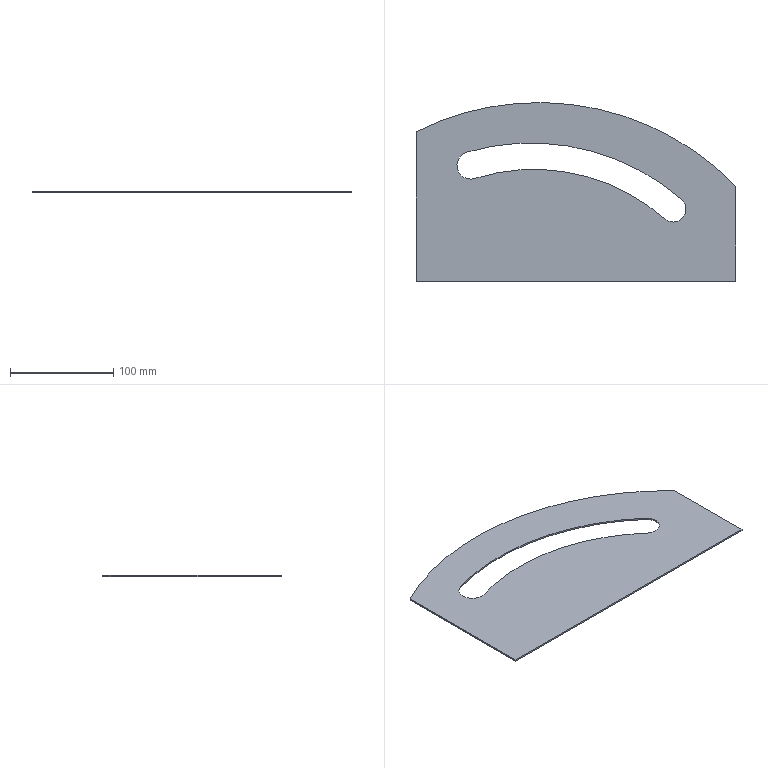Part | STEP file | DEWALT-DWE7492-B22 | 1 solid | 10 faces | box 310 x 173.249 x 1.5 mm | volume 62971 mm3 | cylinder 5 | plane 5 | commonest cylinder face diameters 25.007 x1 26.668 x1 381.573 x1 444.713 x1 530 x1
STEP:
#1=CARTESIAN_POINT('',(0.,0.,0.));
#2=DIRECTION('',(0.,0.,1.));
#3=DIRECTION('',(1.,0.,0.));
#4=AXIS2_PLACEMENT_3D('',#1,#2,#3);
#5=CARTESIAN_POINT('',(56.954,99.676,1.5));
#6=VERTEX_POINT('',#5);
#7=CARTESIAN_POINT('',(56.954,99.676,0.));
#8=VERTEX_POINT('',#7);
#9=CARTESIAN_POINT('',(56.954,99.676,1.5));
#10=DIRECTION('',(0.,0.,-1.));
#11=VECTOR('',#10,1.);
#12=LINE('',#9,#11);
#13=CARTESIAN_POINT('',(52.938,112.391,1.5));
#14=DIRECTION('',(0.,0.,-1.));
#15=DIRECTION('',(-1.,0.,0.));
#16=AXIS2_PLACEMENT_3D('',#13,#14,#15);
#17=CYLINDRICAL_SURFACE('',#16,13.334);
#18=CARTESIAN_POINT('',(4.406,0.));
#19=DIRECTION('',(0.,1.));
#20=VECTOR('',#19,1.);
#21=LINE('',#18,#20);
#22=(GEOMETRIC_REPRESENTATION_CONTEXT(2)PARAMETRIC_REPRESENTATION_CONTEXT()REPRESENTATION_CONTEXT('',''));
#23=DEFINITIONAL_REPRESENTATION('',(#21),#22);
#24=PCURVE('',#17,#23);
#25=CARTESIAN_POINT('',(114.412,-82.252,1.5));
#26=DIRECTION('',(0.,0.,-1.));
#27=DIRECTION('',(-1.,0.,0.));
#28=AXIS2_PLACEMENT_3D('',#25,#26,#27);
#29=CYLINDRICAL_SURFACE('',#28,190.787);
#30=CARTESIAN_POINT('',(1.265,0.));
#31=DIRECTION('',(0.,1.));
#32=VECTOR('',#31,1.);
#33=LINE('',#30,#32);
#34=(GEOMETRIC_REPRESENTATION_CONTEXT(2)PARAMETRIC_REPRESENTATION_CONTEXT()REPRESENTATION_CONTEXT('',''));
#35=DEFINITIONAL_REPRESENTATION('',(#33),#34);
#36=PCURVE('',#29,#35);
#37=SURFACE_CURVE('',#12,(#24,#36),.PCURVE_S1.);
#38=EDGE_CURVE('',#6,#8,#37,.T.);
#39=ORIENTED_EDGE('',*,*,#38,.F.);
#40=CARTESIAN_POINT('',(49.212,125.194,1.5));
#41=VERTEX_POINT('',#40);
#42=CARTESIAN_POINT('',(52.938,112.391,1.5));
#43=DIRECTION('',(0.,0.,-1.));
#44=DIRECTION('',(1.,0.,0.));
#45=AXIS2_PLACEMENT_3D('',#42,#43,#44);
#46=CIRCLE('',#45,13.334);
#47=CARTESIAN_POINT('',(3.142,0.));
#48=DIRECTION('',(1.,0.));
#49=VECTOR('',#48,1.);
#50=LINE('',#47,#49);
#51=(GEOMETRIC_REPRESENTATION_CONTEXT(2)PARAMETRIC_REPRESENTATION_CONTEXT()REPRESENTATION_CONTEXT('',''));
#52=DEFINITIONAL_REPRESENTATION('',(#50),#51);
#53=PCURVE('',#17,#52);
#54=CARTESIAN_POINT('',(119.054,-91.751,1.5));
#55=DIRECTION('',(0.,0.,-1.));
#56=DIRECTION('',(-1.,0.,0.));
#57=AXIS2_PLACEMENT_3D('',#54,#55,#56);
#58=PLANE('',#57);
#59=CARTESIAN_POINT('',(66.116,204.143));
#60=DIRECTION('',(-1.,0.));
#61=AXIS2_PLACEMENT_2D('',#59,#60);
#62=CIRCLE('',#61,13.334);
#63=(GEOMETRIC_REPRESENTATION_CONTEXT(2)PARAMETRIC_REPRESENTATION_CONTEXT()REPRESENTATION_CONTEXT('',''));
#64=DEFINITIONAL_REPRESENTATION('',(#62),#63);
#65=PCURVE('',#58,#64);
#66=SURFACE_CURVE('',#46,(#53,#65),.PCURVE_S1.);
#67=EDGE_CURVE('',#6,#41,#66,.T.);
#68=ORIENTED_EDGE('',*,*,#67,.T.);
#69=CARTESIAN_POINT('',(49.212,125.194,0.));
#70=VERTEX_POINT('',#69);
#71=CARTESIAN_POINT('',(49.212,125.194,1.5));
#72=DIRECTION('',(0.,0.,-1.));
#73=VECTOR('',#72,1.);
#74=LINE('',#71,#73);
#75=CARTESIAN_POINT('',(7.571,0.));
#76=DIRECTION('',(0.,1.));
#77=VECTOR('',#76,1.);
#78=LINE('',#75,#77);
#79=(GEOMETRIC_REPRESENTATION_CONTEXT(2)PARAMETRIC_REPRESENTATION_CONTEXT()REPRESENTATION_CONTEXT('',''));
#80=DEFINITIONAL_REPRESENTATION('',(#78),#79);
#81=PCURVE('',#17,#80);
#82=CARTESIAN_POINT('',(111.356,-88.302,1.5));
#83=DIRECTION('',(0.,0.,-1.));
#84=DIRECTION('',(-1.,0.,0.));
#85=AXIS2_PLACEMENT_3D('',#82,#83,#84);
#86=CYLINDRICAL_SURFACE('',#85,222.357);
#87=CARTESIAN_POINT('',(1.288,0.));
#88=DIRECTION('',(0.,1.));
#89=VECTOR('',#88,1.);
#90=LINE('',#87,#89);
#91=(GEOMETRIC_REPRESENTATION_CONTEXT(2)PARAMETRIC_REPRESENTATION_CONTEXT()REPRESENTATION_CONTEXT('',''));
#92=DEFINITIONAL_REPRESENTATION('',(#90),#91);
#93=PCURVE('',#86,#92);
#94=SURFACE_CURVE('',#74,(#81,#93),.PCURVE_S1.);
#95=EDGE_CURVE('',#41,#70,#94,.T.);
#96=ORIENTED_EDGE('',*,*,#95,.T.);
#97=CARTESIAN_POINT('',(52.938,112.391,0.));
#98=DIRECTION('',(0.,0.,-1.));
#99=DIRECTION('',(1.,0.,0.));
#100=AXIS2_PLACEMENT_3D('',#97,#98,#99);
#101=CIRCLE('',#100,13.334);
#102=CARTESIAN_POINT('',(3.142,1.5));
#103=DIRECTION('',(1.,0.));
#104=VECTOR('',#103,1.);
#105=LINE('',#102,#104);
#106=(GEOMETRIC_REPRESENTATION_CONTEXT(2)PARAMETRIC_REPRESENTATION_CONTEXT()REPRESENTATION_CONTEXT('',''));
#107=DEFINITIONAL_REPRESENTATION('',(#105),#106);
#108=PCURVE('',#17,#107);
#109=CARTESIAN_POINT('',(119.054,-91.751,0.));
#110=DIRECTION('',(0.,0.,-1.));
#111=DIRECTION('',(-1.,0.,0.));
#112=AXIS2_PLACEMENT_3D('',#109,#110,#111);
#113=PLANE('',#112);
#114=CARTESIAN_POINT('',(66.116,204.143));
#115=DIRECTION('',(-1.,0.));
#116=AXIS2_PLACEMENT_2D('',#114,#115);
#117=CIRCLE('',#116,13.334);
#118=(GEOMETRIC_REPRESENTATION_CONTEXT(2)PARAMETRIC_REPRESENTATION_CONTEXT()REPRESENTATION_CONTEXT('',''));
#119=DEFINITIONAL_REPRESENTATION('',(#117),#118);
#120=PCURVE('',#113,#119);
#121=SURFACE_CURVE('',#101,(#108,#120),.PCURVE_S1.);
#122=EDGE_CURVE('',#8,#70,#121,.T.);
#123=ORIENTED_EDGE('',*,*,#122,.F.);
#124=EDGE_LOOP('',(#39,#68,#96,#123));
#125=FACE_BOUND('',#124,.F.);
#126=ADVANCED_FACE('',(#125),#17,.F.);
#127=CARTESIAN_POINT('',(240.815,60.652,0.));
#128=VERTEX_POINT('',#127);
#129=CARTESIAN_POINT('',(114.412,-82.252,0.));
#130=DIRECTION('',(0.,0.,1.));
#131=DIRECTION('',(1.,0.,0.));
#132=AXIS2_PLACEMENT_3D('',#129,#130,#131);
#133=CIRCLE('',#132,190.787);
#134=CARTESIAN_POINT('',(3.142,1.5));
#135=DIRECTION('',(-1.,0.));
#136=VECTOR('',#135,1.);
#137=LINE('',#134,#136);
#138=(GEOMETRIC_REPRESENTATION_CONTEXT(2)PARAMETRIC_REPRESENTATION_CONTEXT()REPRESENTATION_CONTEXT('',''));
#139=DEFINITIONAL_REPRESENTATION('',(#137),#138);
#140=PCURVE('',#29,#139);
#141=CARTESIAN_POINT('',(-186.145,9.499));
#142=CARTESIAN_POINT('',(-186.145,339.951));
#143=CARTESIAN_POINT('',(100.035,174.725));
#144=CARTESIAN_POINT('',(386.215,9.499));
#145=CARTESIAN_POINT('',(100.035,-155.727));
#146=CARTESIAN_POINT('',(-186.145,-320.953));
#147=CARTESIAN_POINT('',(-186.145,9.499));
#148=(BOUNDED_CURVE()B_SPLINE_CURVE(2,(#141,#142,#143,#144,#145,#146,#147),.UNSPECIFIED.,.T.,.F.)B_SPLINE_CURVE_WITH_KNOTS((1,2,2,2,2,1),(-2.094,0.,2.094,4.189,6.283,8.378),.UNSPECIFIED.)CURVE()GEOMETRIC_REPRESENTATION_ITEM()RATIONAL_B_SPLINE_CURVE((1.,0.5,1.,0.5,1.,0.5,1.))REPRESENTATION_ITEM(''));
#149=(GEOMETRIC_REPRESENTATION_CONTEXT(2)PARAMETRIC_REPRESENTATION_CONTEXT()REPRESENTATION_CONTEXT('',''));
#150=DEFINITIONAL_REPRESENTATION('',(#148),#149);
#151=PCURVE('',#113,#150);
#152=SURFACE_CURVE('',#133,(#140,#151),.PCURVE_S1.);
#153=EDGE_CURVE('',#128,#8,#152,.T.);
#154=ORIENTED_EDGE('',*,*,#153,.T.);
#155=ORIENTED_EDGE('',*,*,#38,.F.);
#156=CARTESIAN_POINT('',(240.815,60.652,1.5));
#157=VERTEX_POINT('',#156);
#158=CARTESIAN_POINT('',(114.412,-82.252,1.5));
#159=DIRECTION('',(0.,0.,1.));
#160=DIRECTION('',(1.,0.,0.));
#161=AXIS2_PLACEMENT_3D('',#158,#159,#160);
#162=CIRCLE('',#161,190.787);
#163=CARTESIAN_POINT('',(3.142,0.));
#164=DIRECTION('',(-1.,0.));
#165=VECTOR('',#164,1.);
#166=LINE('',#163,#165);
#167=(GEOMETRIC_REPRESENTATION_CONTEXT(2)PARAMETRIC_REPRESENTATION_CONTEXT()REPRESENTATION_CONTEXT('',''));
#168=DEFINITIONAL_REPRESENTATION('',(#166),#167);
#169=PCURVE('',#29,#168);
#170=CARTESIAN_POINT('',(-186.145,9.499));
#171=CARTESIAN_POINT('',(-186.145,339.951));
#172=CARTESIAN_POINT('',(100.035,174.725));
#173=CARTESIAN_POINT('',(386.215,9.499));
#174=CARTESIAN_POINT('',(100.035,-155.727));
#175=CARTESIAN_POINT('',(-186.145,-320.953));
#176=CARTESIAN_POINT('',(-186.145,9.499));
#177=(BOUNDED_CURVE()B_SPLINE_CURVE(2,(#170,#171,#172,#173,#174,#175,#176),.UNSPECIFIED.,.T.,.F.)B_SPLINE_CURVE_WITH_KNOTS((1,2,2,2,2,1),(-2.094,0.,2.094,4.189,6.283,8.378),.UNSPECIFIED.)CURVE()GEOMETRIC_REPRESENTATION_ITEM()RATIONAL_B_SPLINE_CURVE((1.,0.5,1.,0.5,1.,0.5,1.))REPRESENTATION_ITEM(''));
#178=(GEOMETRIC_REPRESENTATION_CONTEXT(2)PARAMETRIC_REPRESENTATION_CONTEXT()REPRESENTATION_CONTEXT('',''));
#179=DEFINITIONAL_REPRESENTATION('',(#177),#178);
#180=PCURVE('',#58,#179);
#181=SURFACE_CURVE('',#162,(#169,#180),.PCURVE_S1.);
#182=EDGE_CURVE('',#157,#6,#181,.T.);
#183=ORIENTED_EDGE('',*,*,#182,.F.);
#184=CARTESIAN_POINT('',(240.815,60.652,1.5));
#185=DIRECTION('',(0.,0.,-1.));
#186=VECTOR('',#185,1.);
#187=LINE('',#184,#186);
#188=CARTESIAN_POINT('',(2.295,0.));
#189=DIRECTION('',(0.,1.));
#190=VECTOR('',#189,1.);
#191=LINE('',#188,#190);
#192=(GEOMETRIC_REPRESENTATION_CONTEXT(2)PARAMETRIC_REPRESENTATION_CONTEXT()REPRESENTATION_CONTEXT('',''));
#193=DEFINITIONAL_REPRESENTATION('',(#191),#192);
#194=PCURVE('',#29,#193);
#195=CARTESIAN_POINT('',(249.099,70.018,1.5));
#196=DIRECTION('',(0.,0.,-1.));
#197=DIRECTION('',(-1.,0.,0.));
#198=AXIS2_PLACEMENT_3D('',#195,#196,#197);
#199=CYLINDRICAL_SURFACE('',#198,12.504);
#200=CARTESIAN_POINT('',(5.437,0.));
#201=DIRECTION('',(0.,1.));
#202=VECTOR('',#201,1.);
#203=LINE('',#200,#202);
#204=(GEOMETRIC_REPRESENTATION_CONTEXT(2)PARAMETRIC_REPRESENTATION_CONTEXT()REPRESENTATION_CONTEXT('',''));
#205=DEFINITIONAL_REPRESENTATION('',(#203),#204);
#206=PCURVE('',#199,#205);
#207=SURFACE_CURVE('',#187,(#194,#206),.PCURVE_S1.);
#208=EDGE_CURVE('',#157,#128,#207,.T.);
#209=ORIENTED_EDGE('',*,*,#208,.T.);
#210=EDGE_LOOP('',(#154,#155,#183,#209));
#211=FACE_BOUND('',#210,.T.);
#212=ADVANCED_FACE('',(#211),#29,.T.);
#213=CARTESIAN_POINT('',(257.306,79.451,1.5));
#214=VERTEX_POINT('',#213);
#215=CARTESIAN_POINT('',(257.306,79.451,0.));
#216=VERTEX_POINT('',#215);
#217=CARTESIAN_POINT('',(257.306,79.451,1.5));
#218=DIRECTION('',(0.,0.,-1.));
#219=VECTOR('',#218,1.);
#220=LINE('',#217,#219);
#221=CARTESIAN_POINT('',(2.287,0.));
#222=DIRECTION('',(0.,1.));
#223=VECTOR('',#222,1.);
#224=LINE('',#221,#223);
#225=(GEOMETRIC_REPRESENTATION_CONTEXT(2)PARAMETRIC_REPRESENTATION_CONTEXT()REPRESENTATION_CONTEXT('',''));
#226=DEFINITIONAL_REPRESENTATION('',(#224),#225);
#227=PCURVE('',#199,#226);
#228=CARTESIAN_POINT('',(2.287,0.));
#229=DIRECTION('',(0.,1.));
#230=VECTOR('',#229,1.);
#231=LINE('',#228,#230);
#232=(GEOMETRIC_REPRESENTATION_CONTEXT(2)PARAMETRIC_REPRESENTATION_CONTEXT()REPRESENTATION_CONTEXT('',''));
#233=DEFINITIONAL_REPRESENTATION('',(#231),#232);
#234=PCURVE('',#86,#233);
#235=SURFACE_CURVE('',#220,(#227,#234),.PCURVE_S1.);
#236=EDGE_CURVE('',#214,#216,#235,.T.);
#237=ORIENTED_EDGE('',*,*,#236,.F.);
#238=CARTESIAN_POINT('',(249.099,70.018,1.5));
#239=DIRECTION('',(0.,0.,-1.));
#240=DIRECTION('',(-1.,0.,0.));
#241=AXIS2_PLACEMENT_3D('',#238,#239,#240);
#242=CIRCLE('',#241,12.504);
#243=CARTESIAN_POINT('',(0.,0.));
#244=DIRECTION('',(1.,0.));
#245=VECTOR('',#244,1.);
#246=LINE('',#243,#245);
#247=(GEOMETRIC_REPRESENTATION_CONTEXT(2)PARAMETRIC_REPRESENTATION_CONTEXT()REPRESENTATION_CONTEXT('',''));
#248=DEFINITIONAL_REPRESENTATION('',(#246),#247);
#249=PCURVE('',#199,#248);
#250=CARTESIAN_POINT('',(-130.045,161.769));
#251=DIRECTION('',(1.,0.));
#252=AXIS2_PLACEMENT_2D('',#250,#251);
#253=CIRCLE('',#252,12.504);
#254=(GEOMETRIC_REPRESENTATION_CONTEXT(2)PARAMETRIC_REPRESENTATION_CONTEXT()REPRESENTATION_CONTEXT('',''));
#255=DEFINITIONAL_REPRESENTATION('',(#253),#254);
#256=PCURVE('',#58,#255);
#257=SURFACE_CURVE('',#242,(#249,#256),.PCURVE_S1.);
#258=EDGE_CURVE('',#214,#157,#257,.T.);
#259=ORIENTED_EDGE('',*,*,#258,.T.);
#260=ORIENTED_EDGE('',*,*,#208,.T.);
#261=CARTESIAN_POINT('',(249.099,70.018,0.));
#262=DIRECTION('',(0.,0.,-1.));
#263=DIRECTION('',(-1.,0.,0.));
#264=AXIS2_PLACEMENT_3D('',#261,#262,#263);
#265=CIRCLE('',#264,12.504);
#266=CARTESIAN_POINT('',(0.,1.5));
#267=DIRECTION('',(1.,0.));
#268=VECTOR('',#267,1.);
#269=LINE('',#266,#268);
#270=(GEOMETRIC_REPRESENTATION_CONTEXT(2)PARAMETRIC_REPRESENTATION_CONTEXT()REPRESENTATION_CONTEXT('',''));
#271=DEFINITIONAL_REPRESENTATION('',(#269),#270);
#272=PCURVE('',#199,#271);
#273=CARTESIAN_POINT('',(-130.045,161.769));
#274=DIRECTION('',(1.,0.));
#275=AXIS2_PLACEMENT_2D('',#273,#274);
#276=CIRCLE('',#275,12.504);
#277=(GEOMETRIC_REPRESENTATION_CONTEXT(2)PARAMETRIC_REPRESENTATION_CONTEXT()REPRESENTATION_CONTEXT('',''));
#278=DEFINITIONAL_REPRESENTATION('',(#276),#277);
#279=PCURVE('',#113,#278);
#280=SURFACE_CURVE('',#265,(#272,#279),.PCURVE_S1.);
#281=EDGE_CURVE('',#216,#128,#280,.T.);
#282=ORIENTED_EDGE('',*,*,#281,.F.);
#283=EDGE_LOOP('',(#237,#259,#260,#282));
#284=FACE_BOUND('',#283,.F.);
#285=ADVANCED_FACE('',(#284),#199,.F.);
#286=CARTESIAN_POINT('',(310.,0.,0.));
#287=VERTEX_POINT('',#286);
#288=CARTESIAN_POINT('',(0.,0.,0.));
#289=VERTEX_POINT('',#288);
#290=CARTESIAN_POINT('',(310.,0.,0.));
#291=DIRECTION('',(-1.,0.,0.));
#292=VECTOR('',#291,1.);
#293=LINE('',#290,#292);
#294=CARTESIAN_POINT('',(310.,0.,1.5));
#295=DIRECTION('',(0.,-1.,0.));
#296=DIRECTION('',(0.,0.,-1.));
#297=AXIS2_PLACEMENT_3D('',#294,#295,#296);
#298=PLANE('',#297);
#299=CARTESIAN_POINT('',(1.5,0.));
#300=DIRECTION('',(0.,-1.));
#301=VECTOR('',#300,1.);
#302=LINE('',#299,#301);
#303=(GEOMETRIC_REPRESENTATION_CONTEXT(2)PARAMETRIC_REPRESENTATION_CONTEXT()REPRESENTATION_CONTEXT('',''));
#304=DEFINITIONAL_REPRESENTATION('',(#302),#303);
#305=PCURVE('',#298,#304);
#306=CARTESIAN_POINT('',(-190.946,91.751));
#307=DIRECTION('',(1.,0.));
#308=VECTOR('',#307,1.);
#309=LINE('',#306,#308);
#310=(GEOMETRIC_REPRESENTATION_CONTEXT(2)PARAMETRIC_REPRESENTATION_CONTEXT()REPRESENTATION_CONTEXT('',''));
#311=DEFINITIONAL_REPRESENTATION('',(#309),#310);
#312=PCURVE('',#113,#311);
#313=SURFACE_CURVE('',#293,(#305,#312),.PCURVE_S1.);
#314=EDGE_CURVE('',#287,#289,#313,.T.);
#315=ORIENTED_EDGE('',*,*,#314,.F.);
#316=CARTESIAN_POINT('',(310.,0.,1.5));
#317=VERTEX_POINT('',#316);
#318=CARTESIAN_POINT('',(310.,0.,1.5));
#319=DIRECTION('',(0.,0.,-1.));
#320=VECTOR('',#319,1.);
#321=LINE('',#318,#320);
#322=CARTESIAN_POINT('',(0.,0.));
#323=DIRECTION('',(1.,0.));
#324=VECTOR('',#323,1.);
#325=LINE('',#322,#324);
#326=(GEOMETRIC_REPRESENTATION_CONTEXT(2)PARAMETRIC_REPRESENTATION_CONTEXT()REPRESENTATION_CONTEXT('',''));
#327=DEFINITIONAL_REPRESENTATION('',(#325),#326);
#328=PCURVE('',#298,#327);
#329=CARTESIAN_POINT('',(310.,92.,1.5));
#330=DIRECTION('',(1.,0.,0.));
#331=DIRECTION('',(0.,0.,-1.));
#332=AXIS2_PLACEMENT_3D('',#329,#330,#331);
#333=PLANE('',#332);
#334=CARTESIAN_POINT('',(0.,-92.));
#335=DIRECTION('',(1.,0.));
#336=VECTOR('',#335,1.);
#337=LINE('',#334,#336);
#338=(GEOMETRIC_REPRESENTATION_CONTEXT(2)PARAMETRIC_REPRESENTATION_CONTEXT()REPRESENTATION_CONTEXT('',''));
#339=DEFINITIONAL_REPRESENTATION('',(#337),#338);
#340=PCURVE('',#333,#339);
#341=SURFACE_CURVE('',#321,(#328,#340),.PCURVE_S1.);
#342=EDGE_CURVE('',#317,#287,#341,.T.);
#343=ORIENTED_EDGE('',*,*,#342,.F.);
#344=CARTESIAN_POINT('',(0.,0.,1.5));
#345=VERTEX_POINT('',#344);
#346=CARTESIAN_POINT('',(310.,0.,1.5));
#347=DIRECTION('',(-1.,0.,0.));
#348=VECTOR('',#347,1.);
#349=LINE('',#346,#348);
#350=CARTESIAN_POINT('',(0.,0.));
#351=DIRECTION('',(0.,-1.));
#352=VECTOR('',#351,1.);
#353=LINE('',#350,#352);
#354=(GEOMETRIC_REPRESENTATION_CONTEXT(2)PARAMETRIC_REPRESENTATION_CONTEXT()REPRESENTATION_CONTEXT('',''));
#355=DEFINITIONAL_REPRESENTATION('',(#353),#354);
#356=PCURVE('',#298,#355);
#357=CARTESIAN_POINT('',(-190.946,91.751));
#358=DIRECTION('',(1.,0.));
#359=VECTOR('',#358,1.);
#360=LINE('',#357,#359);
#361=(GEOMETRIC_REPRESENTATION_CONTEXT(2)PARAMETRIC_REPRESENTATION_CONTEXT()REPRESENTATION_CONTEXT('',''));
#362=DEFINITIONAL_REPRESENTATION('',(#360),#361);
#363=PCURVE('',#58,#362);
#364=SURFACE_CURVE('',#349,(#356,#363),.PCURVE_S1.);
#365=EDGE_CURVE('',#317,#345,#364,.T.);
#366=ORIENTED_EDGE('',*,*,#365,.T.);
#367=CARTESIAN_POINT('',(0.,0.,1.5));
#368=DIRECTION('',(0.,0.,-1.));
#369=VECTOR('',#368,1.);
#370=LINE('',#367,#369);
#371=CARTESIAN_POINT('',(0.,-310.));
#372=DIRECTION('',(1.,0.));
#373=VECTOR('',#372,1.);
#374=LINE('',#371,#373);
#375=(GEOMETRIC_REPRESENTATION_CONTEXT(2)PARAMETRIC_REPRESENTATION_CONTEXT()REPRESENTATION_CONTEXT('',''));
#376=DEFINITIONAL_REPRESENTATION('',(#374),#375);
#377=PCURVE('',#298,#376);
#378=CARTESIAN_POINT('',(0.,0.,1.5));
#379=DIRECTION('',(-1.,0.,0.));
#380=DIRECTION('',(0.,0.,1.));
#381=AXIS2_PLACEMENT_3D('',#378,#379,#380);
#382=PLANE('',#381);
#383=CARTESIAN_POINT('',(0.,0.));
#384=DIRECTION('',(-1.,0.));
#385=VECTOR('',#384,1.);
#386=LINE('',#383,#385);
#387=(GEOMETRIC_REPRESENTATION_CONTEXT(2)PARAMETRIC_REPRESENTATION_CONTEXT()REPRESENTATION_CONTEXT('',''));
#388=DEFINITIONAL_REPRESENTATION('',(#386),#387);
#389=PCURVE('',#382,#388);
#390=SURFACE_CURVE('',#370,(#377,#389),.PCURVE_S1.);
#391=EDGE_CURVE('',#345,#289,#390,.T.);
#392=ORIENTED_EDGE('',*,*,#391,.T.);
#393=EDGE_LOOP('',(#315,#343,#366,#392));
#394=FACE_BOUND('',#393,.T.);
#395=ADVANCED_FACE('',(#394),#298,.T.);
#396=CARTESIAN_POINT('',(0.,145.,0.));
#397=VERTEX_POINT('',#396);
#398=CARTESIAN_POINT('',(0.,0.,0.));
#399=DIRECTION('',(0.,1.,0.));
#400=VECTOR('',#399,1.);
#401=LINE('',#398,#400);
#402=CARTESIAN_POINT('',(-1.5,0.));
#403=DIRECTION('',(0.,1.));
#404=VECTOR('',#403,1.);
#405=LINE('',#402,#404);
#406=(GEOMETRIC_REPRESENTATION_CONTEXT(2)PARAMETRIC_REPRESENTATION_CONTEXT()REPRESENTATION_CONTEXT('',''));
#407=DEFINITIONAL_REPRESENTATION('',(#405),#406);
#408=PCURVE('',#382,#407);
#409=CARTESIAN_POINT('',(119.054,91.751));
#410=DIRECTION('',(0.,1.));
#411=VECTOR('',#410,1.);
#412=LINE('',#409,#411);
#413=(GEOMETRIC_REPRESENTATION_CONTEXT(2)PARAMETRIC_REPRESENTATION_CONTEXT()REPRESENTATION_CONTEXT('',''));
#414=DEFINITIONAL_REPRESENTATION('',(#412),#413);
#415=PCURVE('',#113,#414);
#416=SURFACE_CURVE('',#401,(#408,#415),.PCURVE_S1.);
#417=EDGE_CURVE('',#289,#397,#416,.T.);
#418=ORIENTED_EDGE('',*,*,#417,.F.);
#419=ORIENTED_EDGE('',*,*,#391,.F.);
#420=CARTESIAN_POINT('',(0.,145.,1.5));
#421=VERTEX_POINT('',#420);
#422=CARTESIAN_POINT('',(0.,0.,1.5));
#423=DIRECTION('',(0.,1.,0.));
#424=VECTOR('',#423,1.);
#425=LINE('',#422,#424);
#426=CARTESIAN_POINT('',(0.,0.));
#427=DIRECTION('',(0.,1.));
#428=VECTOR('',#427,1.);
#429=LINE('',#426,#428);
#430=(GEOMETRIC_REPRESENTATION_CONTEXT(2)PARAMETRIC_REPRESENTATION_CONTEXT()REPRESENTATION_CONTEXT('',''));
#431=DEFINITIONAL_REPRESENTATION('',(#429),#430);
#432=PCURVE('',#382,#431);
#433=CARTESIAN_POINT('',(119.054,91.751));
#434=DIRECTION('',(0.,1.));
#435=VECTOR('',#434,1.);
#436=LINE('',#433,#435);
#437=(GEOMETRIC_REPRESENTATION_CONTEXT(2)PARAMETRIC_REPRESENTATION_CONTEXT()REPRESENTATION_CONTEXT('',''));
#438=DEFINITIONAL_REPRESENTATION('',(#436),#437);
#439=PCURVE('',#58,#438);
#440=SURFACE_CURVE('',#425,(#432,#439),.PCURVE_S1.);
#441=EDGE_CURVE('',#345,#421,#440,.T.);
#442=ORIENTED_EDGE('',*,*,#441,.T.);
#443=CARTESIAN_POINT('',(0.,145.,1.5));
#444=DIRECTION('',(0.,0.,-1.));
#445=VECTOR('',#444,1.);
#446=LINE('',#443,#445);
#447=CARTESIAN_POINT('',(0.,145.));
#448=DIRECTION('',(-1.,0.));
#449=VECTOR('',#448,1.);
#450=LINE('',#447,#449);
#451=(GEOMETRIC_REPRESENTATION_CONTEXT(2)PARAMETRIC_REPRESENTATION_CONTEXT()REPRESENTATION_CONTEXT('',''));
#452=DEFINITIONAL_REPRESENTATION('',(#450),#451);
#453=PCURVE('',#382,#452);
#454=CARTESIAN_POINT('',(119.054,-91.751,1.5));
#455=DIRECTION('',(0.,0.,-1.));
#456=DIRECTION('',(-1.,0.,0.));
#457=AXIS2_PLACEMENT_3D('',#454,#455,#456);
#458=CYLINDRICAL_SURFACE('',#457,265.);
#459=CARTESIAN_POINT('',(1.105,0.));
#460=DIRECTION('',(0.,1.));
#461=VECTOR('',#460,1.);
#462=LINE('',#459,#461);
#463=(GEOMETRIC_REPRESENTATION_CONTEXT(2)PARAMETRIC_REPRESENTATION_CONTEXT()REPRESENTATION_CONTEXT('',''));
#464=DEFINITIONAL_REPRESENTATION('',(#462),#463);
#465=PCURVE('',#458,#464);
#466=SURFACE_CURVE('',#446,(#453,#465),.PCURVE_S1.);
#467=EDGE_CURVE('',#421,#397,#466,.T.);
#468=ORIENTED_EDGE('',*,*,#467,.T.);
#469=EDGE_LOOP('',(#418,#419,#442,#468));
#470=FACE_BOUND('',#469,.T.);
#471=ADVANCED_FACE('',(#470),#382,.T.);
#472=CARTESIAN_POINT('',(310.,92.,0.));
#473=VERTEX_POINT('',#472);
#474=CARTESIAN_POINT('',(119.054,-91.751,0.));
#475=DIRECTION('',(0.,0.,-1.));
#476=DIRECTION('',(1.,0.,0.));
#477=AXIS2_PLACEMENT_3D('',#474,#475,#476);
#478=CIRCLE('',#477,265.);
#479=CARTESIAN_POINT('',(-3.142,1.5));
#480=DIRECTION('',(1.,0.));
#481=VECTOR('',#480,1.);
#482=LINE('',#479,#481);
#483=(GEOMETRIC_REPRESENTATION_CONTEXT(2)PARAMETRIC_REPRESENTATION_CONTEXT()REPRESENTATION_CONTEXT('',''));
#484=DEFINITIONAL_REPRESENTATION('',(#482),#483);
#485=PCURVE('',#458,#484);
#486=CARTESIAN_POINT('',(0.,0.));
#487=DIRECTION('',(-1.,0.));
#488=AXIS2_PLACEMENT_2D('',#486,#487);
#489=CIRCLE('',#488,265.);
#490=(GEOMETRIC_REPRESENTATION_CONTEXT(2)PARAMETRIC_REPRESENTATION_CONTEXT()REPRESENTATION_CONTEXT('',''));
#491=DEFINITIONAL_REPRESENTATION('',(#489),#490);
#492=PCURVE('',#113,#491);
#493=SURFACE_CURVE('',#478,(#485,#492),.PCURVE_S1.);
#494=EDGE_CURVE('',#397,#473,#493,.T.);
#495=ORIENTED_EDGE('',*,*,#494,.F.);
#496=ORIENTED_EDGE('',*,*,#467,.F.);
#497=CARTESIAN_POINT('',(310.,92.,1.5));
#498=VERTEX_POINT('',#497);
#499=CARTESIAN_POINT('',(119.054,-91.751,1.5));
#500=DIRECTION('',(0.,0.,-1.));
#501=DIRECTION('',(1.,0.,0.));
#502=AXIS2_PLACEMENT_3D('',#499,#500,#501);
#503=CIRCLE('',#502,265.);
#504=CARTESIAN_POINT('',(-3.142,0.));
#505=DIRECTION('',(1.,0.));
#506=VECTOR('',#505,1.);
#507=LINE('',#504,#506);
#508=(GEOMETRIC_REPRESENTATION_CONTEXT(2)PARAMETRIC_REPRESENTATION_CONTEXT()REPRESENTATION_CONTEXT('',''));
#509=DEFINITIONAL_REPRESENTATION('',(#507),#508);
#510=PCURVE('',#458,#509);
#511=CARTESIAN_POINT('',(0.,0.));
#512=DIRECTION('',(-1.,0.));
#513=AXIS2_PLACEMENT_2D('',#511,#512);
#514=CIRCLE('',#513,265.);
#515=(GEOMETRIC_REPRESENTATION_CONTEXT(2)PARAMETRIC_REPRESENTATION_CONTEXT()REPRESENTATION_CONTEXT('',''));
#516=DEFINITIONAL_REPRESENTATION('',(#514),#515);
#517=PCURVE('',#58,#516);
#518=SURFACE_CURVE('',#503,(#510,#517),.PCURVE_S1.);
#519=EDGE_CURVE('',#421,#498,#518,.T.);
#520=ORIENTED_EDGE('',*,*,#519,.T.);
#521=CARTESIAN_POINT('',(310.,92.,1.5));
#522=DIRECTION('',(0.,0.,-1.));
#523=VECTOR('',#522,1.);
#524=LINE('',#521,#523);
#525=CARTESIAN_POINT('',(2.375,0.));
#526=DIRECTION('',(0.,1.));
#527=VECTOR('',#526,1.);
#528=LINE('',#525,#527);
#529=(GEOMETRIC_REPRESENTATION_CONTEXT(2)PARAMETRIC_REPRESENTATION_CONTEXT()REPRESENTATION_CONTEXT('',''));
#530=DEFINITIONAL_REPRESENTATION('',(#528),#529);
#531=PCURVE('',#458,#530);
#532=CARTESIAN_POINT('',(0.,0.));
#533=DIRECTION('',(1.,0.));
#534=VECTOR('',#533,1.);
#535=LINE('',#532,#534);
#536=(GEOMETRIC_REPRESENTATION_CONTEXT(2)PARAMETRIC_REPRESENTATION_CONTEXT()REPRESENTATION_CONTEXT('',''));
#537=DEFINITIONAL_REPRESENTATION('',(#535),#536);
#538=PCURVE('',#333,#537);
#539=SURFACE_CURVE('',#524,(#531,#538),.PCURVE_S1.);
#540=EDGE_CURVE('',#498,#473,#539,.T.);
#541=ORIENTED_EDGE('',*,*,#540,.T.);
#542=EDGE_LOOP('',(#495,#496,#520,#541));
#543=FACE_BOUND('',#542,.T.);
#544=ADVANCED_FACE('',(#543),#458,.T.);
#545=CARTESIAN_POINT('',(310.,92.,0.));
#546=DIRECTION('',(0.,-1.,0.));
#547=VECTOR('',#546,1.);
#548=LINE('',#545,#547);
#549=CARTESIAN_POINT('',(1.5,0.));
#550=DIRECTION('',(0.,-1.));
#551=VECTOR('',#550,1.);
#552=LINE('',#549,#551);
#553=(GEOMETRIC_REPRESENTATION_CONTEXT(2)PARAMETRIC_REPRESENTATION_CONTEXT()REPRESENTATION_CONTEXT('',''));
#554=DEFINITIONAL_REPRESENTATION('',(#552),#553);
#555=PCURVE('',#333,#554);
#556=CARTESIAN_POINT('',(-190.946,183.751));
#557=DIRECTION('',(0.,-1.));
#558=VECTOR('',#557,1.);
#559=LINE('',#556,#558);
#560=(GEOMETRIC_REPRESENTATION_CONTEXT(2)PARAMETRIC_REPRESENTATION_CONTEXT()REPRESENTATION_CONTEXT('',''));
#561=DEFINITIONAL_REPRESENTATION('',(#559),#560);
#562=PCURVE('',#113,#561);
#563=SURFACE_CURVE('',#548,(#555,#562),.PCURVE_S1.);
#564=EDGE_CURVE('',#473,#287,#563,.T.);
#565=ORIENTED_EDGE('',*,*,#564,.F.);
#566=ORIENTED_EDGE('',*,*,#540,.F.);
#567=CARTESIAN_POINT('',(310.,92.,1.5));
#568=DIRECTION('',(0.,-1.,0.));
#569=VECTOR('',#568,1.);
#570=LINE('',#567,#569);
#571=CARTESIAN_POINT('',(0.,0.));
#572=DIRECTION('',(0.,-1.));
#573=VECTOR('',#572,1.);
#574=LINE('',#571,#573);
#575=(GEOMETRIC_REPRESENTATION_CONTEXT(2)PARAMETRIC_REPRESENTATION_CONTEXT()REPRESENTATION_CONTEXT('',''));
#576=DEFINITIONAL_REPRESENTATION('',(#574),#575);
#577=PCURVE('',#333,#576);
#578=CARTESIAN_POINT('',(-190.946,183.751));
#579=DIRECTION('',(0.,-1.));
#580=VECTOR('',#579,1.);
#581=LINE('',#578,#580);
#582=(GEOMETRIC_REPRESENTATION_CONTEXT(2)PARAMETRIC_REPRESENTATION_CONTEXT()REPRESENTATION_CONTEXT('',''));
#583=DEFINITIONAL_REPRESENTATION('',(#581),#582);
#584=PCURVE('',#58,#583);
#585=SURFACE_CURVE('',#570,(#577,#584),.PCURVE_S1.);
#586=EDGE_CURVE('',#498,#317,#585,.T.);
#587=ORIENTED_EDGE('',*,*,#586,.T.);
#588=ORIENTED_EDGE('',*,*,#342,.T.);
#589=EDGE_LOOP('',(#565,#566,#587,#588));
#590=FACE_BOUND('',#589,.T.);
#591=ADVANCED_FACE('',(#590),#333,.T.);
#592=ORIENTED_EDGE('',*,*,#95,.F.);
#593=CARTESIAN_POINT('',(111.356,-88.302,1.5));
#594=DIRECTION('',(0.,0.,-1.));
#595=DIRECTION('',(1.,0.,0.));
#596=AXIS2_PLACEMENT_3D('',#593,#594,#595);
#597=CIRCLE('',#596,222.357);
#598=CARTESIAN_POINT('',(-3.142,0.));
#599=DIRECTION('',(1.,0.));
#600=VECTOR('',#599,1.);
#601=LINE('',#598,#600);
#602=(GEOMETRIC_REPRESENTATION_CONTEXT(2)PARAMETRIC_REPRESENTATION_CONTEXT()REPRESENTATION_CONTEXT('',''));
#603=DEFINITIONAL_REPRESENTATION('',(#601),#602);
#604=PCURVE('',#86,#603);
#605=CARTESIAN_POINT('',(7.697,3.449));
#606=DIRECTION('',(-1.,0.));
#607=AXIS2_PLACEMENT_2D('',#605,#606);
#608=CIRCLE('',#607,222.357);
#609=(GEOMETRIC_REPRESENTATION_CONTEXT(2)PARAMETRIC_REPRESENTATION_CONTEXT()REPRESENTATION_CONTEXT('',''));
#610=DEFINITIONAL_REPRESENTATION('',(#608),#609);
#611=PCURVE('',#58,#610);
#612=SURFACE_CURVE('',#597,(#604,#611),.PCURVE_S1.);
#613=EDGE_CURVE('',#41,#214,#612,.T.);
#614=ORIENTED_EDGE('',*,*,#613,.T.);
#615=ORIENTED_EDGE('',*,*,#236,.T.);
#616=CARTESIAN_POINT('',(111.356,-88.302,0.));
#617=DIRECTION('',(0.,0.,-1.));
#618=DIRECTION('',(1.,0.,0.));
#619=AXIS2_PLACEMENT_3D('',#616,#617,#618);
#620=CIRCLE('',#619,222.357);
#621=CARTESIAN_POINT('',(-3.142,1.5));
#622=DIRECTION('',(1.,0.));
#623=VECTOR('',#622,1.);
#624=LINE('',#621,#623);
#625=(GEOMETRIC_REPRESENTATION_CONTEXT(2)PARAMETRIC_REPRESENTATION_CONTEXT()REPRESENTATION_CONTEXT('',''));
#626=DEFINITIONAL_REPRESENTATION('',(#624),#625);
#627=PCURVE('',#86,#626);
#628=CARTESIAN_POINT('',(7.697,3.449));
#629=DIRECTION('',(-1.,0.));
#630=AXIS2_PLACEMENT_2D('',#628,#629);
#631=CIRCLE('',#630,222.357);
#632=(GEOMETRIC_REPRESENTATION_CONTEXT(2)PARAMETRIC_REPRESENTATION_CONTEXT()REPRESENTATION_CONTEXT('',''));
#633=DEFINITIONAL_REPRESENTATION('',(#631),#632);
#634=PCURVE('',#113,#633);
#635=SURFACE_CURVE('',#620,(#627,#634),.PCURVE_S1.);
#636=EDGE_CURVE('',#70,#216,#635,.T.);
#637=ORIENTED_EDGE('',*,*,#636,.F.);
#638=EDGE_LOOP('',(#592,#614,#615,#637));
#639=FACE_BOUND('',#638,.F.);
#640=ADVANCED_FACE('',(#639),#86,.F.);
#641=ORIENTED_EDGE('',*,*,#365,.F.);
#642=ORIENTED_EDGE('',*,*,#586,.F.);
#643=ORIENTED_EDGE('',*,*,#519,.F.);
#644=ORIENTED_EDGE('',*,*,#441,.F.);
#645=EDGE_LOOP('',(#641,#642,#643,#644));
#646=FACE_BOUND('',#645,.T.);
#647=ORIENTED_EDGE('',*,*,#67,.T.);
#648=ORIENTED_EDGE('',*,*,#613,.T.);
#649=ORIENTED_EDGE('',*,*,#258,.T.);
#650=ORIENTED_EDGE('',*,*,#182,.T.);
#651=EDGE_LOOP('',(#647,#648,#649,#650));
#652=FACE_BOUND('',#651,.T.);
#653=ADVANCED_FACE('',(#646,#652),#58,.F.);
#654=ORIENTED_EDGE('',*,*,#314,.T.);
#655=ORIENTED_EDGE('',*,*,#417,.T.);
#656=ORIENTED_EDGE('',*,*,#494,.T.);
#657=ORIENTED_EDGE('',*,*,#564,.T.);
#658=EDGE_LOOP('',(#654,#655,#656,#657));
#659=FACE_BOUND('',#658,.T.);
#660=ORIENTED_EDGE('',*,*,#122,.F.);
#661=ORIENTED_EDGE('',*,*,#153,.F.);
#662=ORIENTED_EDGE('',*,*,#281,.F.);
#663=ORIENTED_EDGE('',*,*,#636,.F.);
#664=EDGE_LOOP('',(#660,#661,#662,#663));
#665=FACE_BOUND('',#664,.T.);
#666=ADVANCED_FACE('',(#659,#665),#113,.T.);
#667=CLOSED_SHELL('',(#126,#212,#285,#395,#471,#544,#591,#640,#653,#666));
#668=MANIFOLD_SOLID_BREP('',#667);
#669=(LENGTH_UNIT()NAMED_UNIT(*)SI_UNIT(.MILLI.,.METRE.));
#670=UNCERTAINTY_MEASURE_WITH_UNIT(LENGTH_MEASURE(0.0000001),#669,'','');
#671=(NAMED_UNIT(*)PLANE_ANGLE_UNIT()SI_UNIT($,.RADIAN.));
#672=(NAMED_UNIT(*)SI_UNIT($,.STERADIAN.)SOLID_ANGLE_UNIT());
#673=(GEOMETRIC_REPRESENTATION_CONTEXT(3)GLOBAL_UNCERTAINTY_ASSIGNED_CONTEXT((#670))GLOBAL_UNIT_ASSIGNED_CONTEXT((#669,#671,#672))REPRESENTATION_CONTEXT('',''));
#674=ADVANCED_BREP_SHAPE_REPRESENTATION('',(#4,#668),#673);